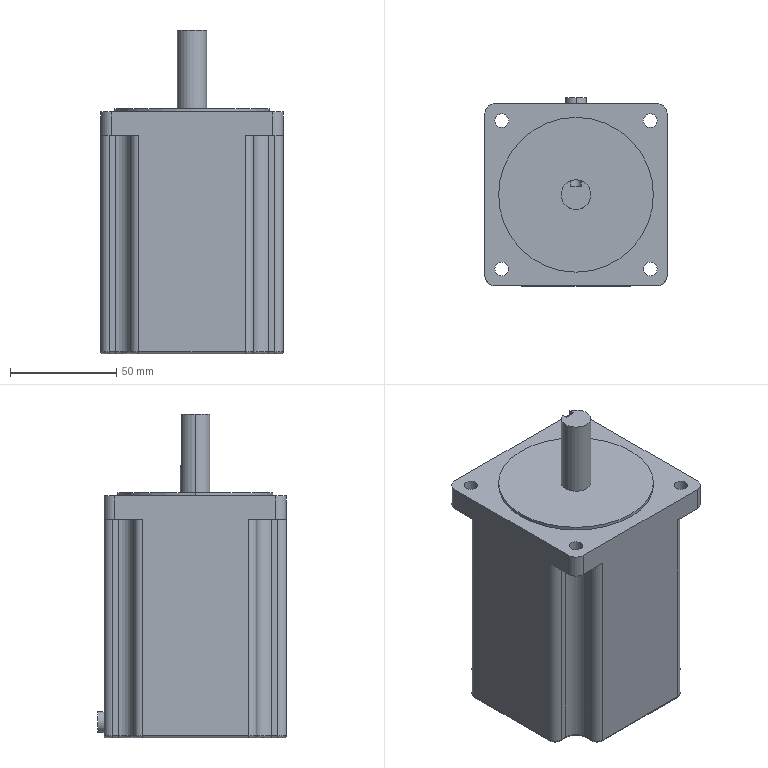Part | STEP file | Stepper Motor 34HS4801D14PJ5 | 1 solid | 79 faces | box 86 x 89 x 152.5 mm | volume 773985 mm3 | cylinder 43 | plane 24 | torus 12 | commonest cylinder face diameters 2 x12 6.5 x8 8 x8 14 x6 10 x4 9.862 x2